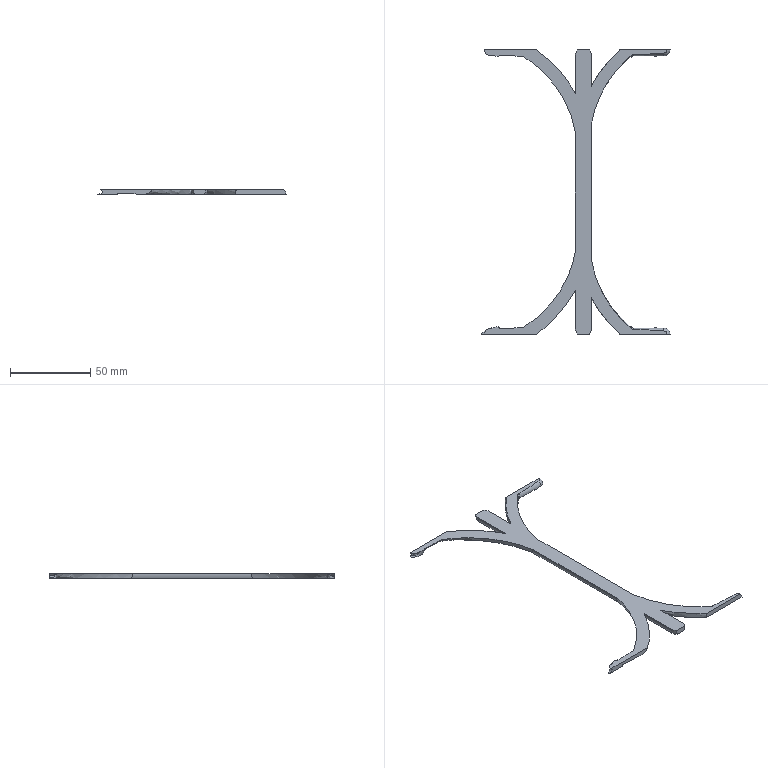Part | STEP file | solid 223 | 1 solid | 54 faces | box 117.1 x 176.873 x 3.297 mm | volume 10209 mm3 | spline 22 | cylinder 12 | plane 12 | sphere 8 | commonest cylinder face diameters 8 x6 10 x6